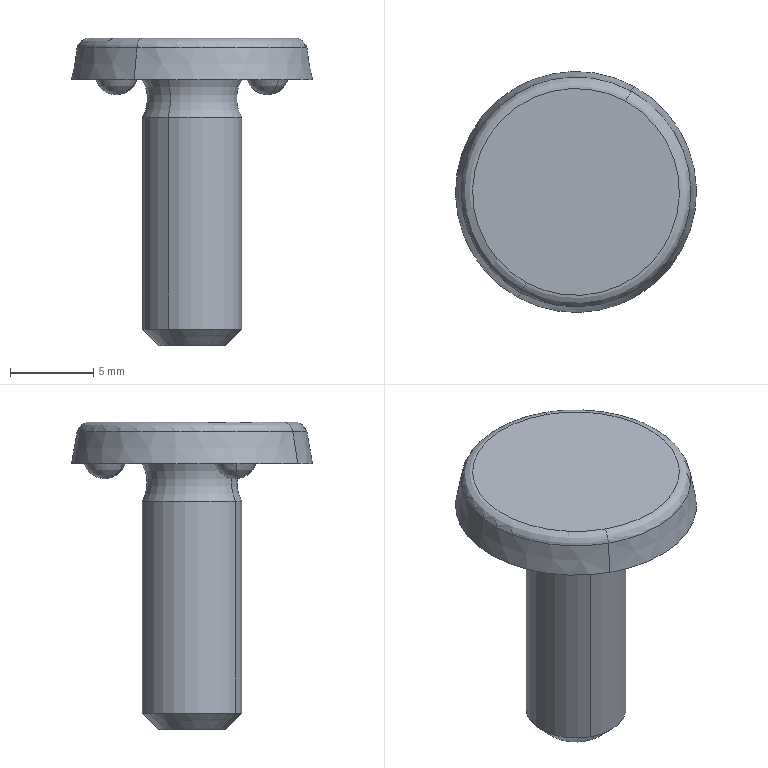Part | STEP file | Q1980616 | 1 solid | 19 faces | box 14.5 x 14.5 x 18.5 mm | volume 828.674 mm3 | sphere 6 | cone 4 | torus 4 | plane 3 | cylinder 2 | commonest cylinder face diameters 6 x2
STEP:
#1=CARTESIAN_POINT('',(4.547,-2.625,-0.9));
#2=VERTEX_POINT('',#1);
#3=CARTESIAN_POINT('',(5.19,-3.681,0.));
#4=VERTEX_POINT('',#3);
#5=CARTESIAN_POINT('',(4.547,-2.625,0.4));
#6=DIRECTION('',(0.854,0.5203,0.));
#7=AXIS2_PLACEMENT_3D('',#5,#6,$);
#8=CIRCLE('',#7,1.3);
#9=EDGE_CURVE('',#2,#4,#8,.F.);
#10=ORIENTED_EDGE('',*,*,#9,.F.);
#11=CARTESIAN_POINT('',(3.903,-1.569,0.));
#12=VERTEX_POINT('',#11);
#13=CARTESIAN_POINT('',(4.547,-2.625,0.4));
#14=DIRECTION('',(-0.854,-0.5203,0.));
#15=AXIS2_PLACEMENT_3D('',#13,#14,$);
#16=CIRCLE('',#15,1.3);
#17=EDGE_CURVE('',#2,#12,#16,.F.);
#18=ORIENTED_EDGE('',*,*,#17,.T.);
#19=CARTESIAN_POINT('',(5.19,-3.681,0.));
#20=CARTESIAN_POINT('',(5.46,-3.517,0.));
#21=CARTESIAN_POINT('',(5.678,-3.266,0.));
#22=CARTESIAN_POINT('',(5.805,-2.951,0.));
#23=CARTESIAN_POINT('',(5.832,-2.453,0.));
#24=CARTESIAN_POINT('',(5.639,-2.013,0.));
#25=CARTESIAN_POINT('',(5.551,-1.877,0.));
#26=CARTESIAN_POINT('',(5.238,-1.532,0.));
#27=CARTESIAN_POINT('',(4.79,-1.354,0.));
#28=CARTESIAN_POINT('',(4.468,-1.333,0.));
#29=CARTESIAN_POINT('',(4.161,-1.411,0.));
#30=CARTESIAN_POINT('',(3.903,-1.569,0.));
#31=B_SPLINE_CURVE_WITH_KNOTS('',5,(#19,#20,#21,#22,#23,#24,#25,#26,#27,#28,#29,#30),.UNSPECIFIED.,.F.,.U.,(6,3,3,6),(0.,2.294,3.444,5.637),.UNSPECIFIED.);
#32=EDGE_CURVE('',#4,#12,#31,.T.);
#33=ORIENTED_EDGE('',*,*,#32,.F.);
#34=EDGE_LOOP('',(#10,#18,#33));
#35=FACE_OUTER_BOUND('',#34,.T.);
#36=CARTESIAN_POINT('',(4.547,-2.625,0.4));
#37=DIRECTION('',(0.,0.,-1.));
#38=DIRECTION('',(0.5203,-0.854,0.));
#39=AXIS2_PLACEMENT_3D('',#36,#37,#38);
#40=SPHERICAL_SURFACE('',#39,1.3);
#41=ADVANCED_FACE('',(#35),#40,.T.);
#42=ORIENTED_EDGE('',*,*,#17,.F.);
#43=ORIENTED_EDGE('',*,*,#9,.T.);
#44=CARTESIAN_POINT('',(5.19,-3.681,0.));
#45=CARTESIAN_POINT('',(4.92,-3.846,0.));
#46=CARTESIAN_POINT('',(4.598,-3.924,0.));
#47=CARTESIAN_POINT('',(4.259,-3.893,0.));
#48=CARTESIAN_POINT('',(3.804,-3.689,0.));
#49=CARTESIAN_POINT('',(3.502,-3.315,0.));
#50=CARTESIAN_POINT('',(3.422,-3.175,0.));
#51=CARTESIAN_POINT('',(3.258,-2.738,0.));
#52=CARTESIAN_POINT('',(3.305,-2.258,0.));
#53=CARTESIAN_POINT('',(3.435,-1.962,0.));
#54=CARTESIAN_POINT('',(3.645,-1.726,0.));
#55=CARTESIAN_POINT('',(3.903,-1.569,0.));
#56=B_SPLINE_CURVE_WITH_KNOTS('',5,(#44,#45,#46,#47,#48,#49,#50,#51,#52,#53,#54,#55),.UNSPECIFIED.,.F.,.U.,(6,3,3,6),(0.,2.294,3.444,5.637),.UNSPECIFIED.);
#57=EDGE_CURVE('',#4,#12,#56,.T.);
#58=ORIENTED_EDGE('',*,*,#57,.T.);
#59=EDGE_LOOP('',(#42,#43,#58));
#60=FACE_OUTER_BOUND('',#59,.T.);
#61=ADVANCED_FACE('',(#60),#40,.T.);
#62=CARTESIAN_POINT('',(-3.476,-6.362,0.));
#63=VERTEX_POINT('',#62);
#64=CARTESIAN_POINT('',(3.476,6.362,0.));
#65=VERTEX_POINT('',#64);
#66=CARTESIAN_POINT('',(0.,0.,0.));
#67=DIRECTION('',(0.,0.,-1.));
#68=AXIS2_PLACEMENT_3D('',#66,#67,$);
#69=CIRCLE('',#68,7.25);
#70=EDGE_CURVE('',#63,#65,#69,.T.);
#71=ORIENTED_EDGE('',*,*,#70,.T.);
#72=CARTESIAN_POINT('',(0.,0.,0.));
#73=DIRECTION('',(0.,0.,-1.));
#74=AXIS2_PLACEMENT_3D('',#72,#73,$);
#75=CIRCLE('',#74,7.25);
#76=EDGE_CURVE('',#65,#63,#75,.T.);
#77=ORIENTED_EDGE('',*,*,#76,.T.);
#78=EDGE_LOOP('',(#71,#77));
#79=FACE_OUTER_BOUND('',#78,.T.);
#80=CARTESIAN_POINT('',(1.438,2.633,0.));
#81=VERTEX_POINT('',#80);
#82=CARTESIAN_POINT('',(-1.438,-2.633,0.));
#83=VERTEX_POINT('',#82);
#84=CARTESIAN_POINT('',(0.,0.,0.));
#85=DIRECTION('',(0.,0.,-1.));
#86=AXIS2_PLACEMENT_3D('',#84,#85,$);
#87=CIRCLE('',#86,3.);
#88=EDGE_CURVE('',#81,#83,#87,.T.);
#89=ORIENTED_EDGE('',*,*,#88,.F.);
#90=CARTESIAN_POINT('',(0.,0.,0.));
#91=DIRECTION('',(0.,0.,-1.));
#92=AXIS2_PLACEMENT_3D('',#90,#91,$);
#93=CIRCLE('',#92,3.);
#94=EDGE_CURVE('',#83,#81,#93,.T.);
#95=ORIENTED_EDGE('',*,*,#94,.F.);
#96=EDGE_LOOP('',(#89,#95));
#97=FACE_BOUND('',#96,.T.);
#98=CARTESIAN_POINT('',(-5.783,-2.654,0.));
#99=VERTEX_POINT('',#98);
#100=CARTESIAN_POINT('',(-3.31,-2.596,0.));
#101=VERTEX_POINT('',#100);
#102=CARTESIAN_POINT('',(-5.783,-2.654,0.));
#103=CARTESIAN_POINT('',(-5.787,-2.497,0.));
#104=CARTESIAN_POINT('',(-5.766,-2.338,0.));
#105=CARTESIAN_POINT('',(-5.719,-2.185,0.));
#106=CARTESIAN_POINT('',(-5.578,-1.897,0.));
#107=CARTESIAN_POINT('',(-5.355,-1.668,0.));
#108=CARTESIAN_POINT('',(-5.225,-1.572,0.));
#109=CARTESIAN_POINT('',(-4.939,-1.425,0.));
#110=CARTESIAN_POINT('',(-4.622,-1.375,0.));
#111=CARTESIAN_POINT('',(-4.46,-1.376,0.));
#112=CARTESIAN_POINT('',(-4.144,-1.429,0.));
#113=CARTESIAN_POINT('',(-3.859,-1.578,0.));
#114=CARTESIAN_POINT('',(-3.73,-1.675,0.));
#115=CARTESIAN_POINT('',(-3.519,-1.896,0.));
#116=CARTESIAN_POINT('',(-3.383,-2.17,0.));
#117=CARTESIAN_POINT('',(-3.338,-2.309,0.));
#118=CARTESIAN_POINT('',(-3.313,-2.452,0.));
#119=CARTESIAN_POINT('',(-3.31,-2.596,0.));
#120=B_SPLINE_CURVE_WITH_KNOTS('',5,(#102,#103,#104,#105,#106,#107,#108,#109,#110,#111,#112,#113,#114,#115,#116,#117,#118,#119),.UNSPECIFIED.,.F.,.U.,(6,3,3,3,3,6),(0.,1.143,2.294,3.444,4.595,5.637),.UNSPECIFIED.);
#121=EDGE_CURVE('',#99,#101,#120,.T.);
#122=ORIENTED_EDGE('',*,*,#121,.F.);
#123=CARTESIAN_POINT('',(-5.783,-2.654,0.));
#124=CARTESIAN_POINT('',(-5.78,-2.812,0.));
#125=CARTESIAN_POINT('',(-5.751,-2.969,0.));
#126=CARTESIAN_POINT('',(-5.697,-3.12,0.));
#127=CARTESIAN_POINT('',(-5.543,-3.4,0.));
#128=CARTESIAN_POINT('',(-5.309,-3.619,0.));
#129=CARTESIAN_POINT('',(-5.174,-3.709,0.));
#130=CARTESIAN_POINT('',(-4.882,-3.842,0.));
#131=CARTESIAN_POINT('',(-4.563,-3.877,0.));
#132=CARTESIAN_POINT('',(-4.402,-3.869,0.));
#133=CARTESIAN_POINT('',(-4.088,-3.801,0.));
#134=CARTESIAN_POINT('',(-3.811,-3.638,0.));
#135=CARTESIAN_POINT('',(-3.686,-3.535,0.));
#136=CARTESIAN_POINT('',(-3.485,-3.304,0.));
#137=CARTESIAN_POINT('',(-3.363,-3.024,0.));
#138=CARTESIAN_POINT('',(-3.324,-2.884,0.));
#139=CARTESIAN_POINT('',(-3.307,-2.74,0.));
#140=CARTESIAN_POINT('',(-3.31,-2.596,0.));
#141=B_SPLINE_CURVE_WITH_KNOTS('',5,(#123,#124,#125,#126,#127,#128,#129,#130,#131,#132,#133,#134,#135,#136,#137,#138,#139,#140),.UNSPECIFIED.,.F.,.U.,(6,3,3,3,3,6),(0.,1.143,2.294,3.444,4.595,5.637),.UNSPECIFIED.);
#142=EDGE_CURVE('',#99,#101,#141,.T.);
#143=ORIENTED_EDGE('',*,*,#142,.T.);
#144=EDGE_LOOP('',(#122,#143));
#145=FACE_BOUND('',#144,.T.);
#146=CARTESIAN_POINT('',(0.593,6.336,0.));
#147=VERTEX_POINT('',#146);
#148=CARTESIAN_POINT('',(-0.593,4.164,0.));
#149=VERTEX_POINT('',#148);
#150=CARTESIAN_POINT('',(0.593,6.336,0.));
#151=CARTESIAN_POINT('',(0.7313,6.26,0.));
#152=CARTESIAN_POINT('',(0.8576,6.162,0.));
#153=CARTESIAN_POINT('',(0.9672,6.045,0.));
#154=CARTESIAN_POINT('',(1.146,5.779,0.));
#155=CARTESIAN_POINT('',(1.233,5.471,0.));
#156=CARTESIAN_POINT('',(1.251,5.311,0.));
#157=CARTESIAN_POINT('',(1.235,4.99,0.));
#158=CARTESIAN_POINT('',(1.12,4.69,0.));
#159=CARTESIAN_POINT('',(1.039,4.551,0.));
#160=CARTESIAN_POINT('',(0.8345,4.303,0.));
#161=CARTESIAN_POINT('',(0.5629,4.131,0.));
#162=CARTESIAN_POINT('',(0.4143,4.068,0.));
#163=CARTESIAN_POINT('',(0.1169,3.995,0.));
#164=CARTESIAN_POINT('',(-0.188,4.015,0.));
#165=CARTESIAN_POINT('',(-0.3307,4.045,0.));
#166=CARTESIAN_POINT('',(-0.4669,4.096,0.));
#167=CARTESIAN_POINT('',(-0.593,4.164,0.));
#168=B_SPLINE_CURVE_WITH_KNOTS('',5,(#150,#151,#152,#153,#154,#155,#156,#157,#158,#159,#160,#161,#162,#163,#164,#165,#166,#167),.UNSPECIFIED.,.F.,.U.,(6,3,3,3,3,6),(0.,1.143,2.294,3.444,4.595,5.637),.UNSPECIFIED.);
#169=EDGE_CURVE('',#147,#149,#168,.T.);
#170=ORIENTED_EDGE('',*,*,#169,.F.);
#171=CARTESIAN_POINT('',(0.593,6.336,0.));
#172=CARTESIAN_POINT('',(0.4547,6.411,0.));
#173=CARTESIAN_POINT('',(0.3043,6.465,0.));
#174=CARTESIAN_POINT('',(0.1466,6.494,0.));
#175=CARTESIAN_POINT('',(-0.1735,6.5,0.));
#176=CARTESIAN_POINT('',(-0.4798,6.407,0.));
#177=CARTESIAN_POINT('',(-0.6246,6.335,0.));
#178=CARTESIAN_POINT('',(-0.8862,6.149,0.));
#179=CARTESIAN_POINT('',(-1.076,5.89,0.));
#180=CARTESIAN_POINT('',(-1.15,5.746,0.));
#181=CARTESIAN_POINT('',(-1.248,5.44,0.));
#182=CARTESIAN_POINT('',(-1.245,5.119,0.));
#183=CARTESIAN_POINT('',(-1.218,4.96,0.));
#184=CARTESIAN_POINT('',(-1.119,4.67,0.));
#185=CARTESIAN_POINT('',(-0.9379,4.424,0.));
#186=CARTESIAN_POINT('',(-0.8353,4.321,0.));
#187=CARTESIAN_POINT('',(-0.7192,4.233,0.));
#188=CARTESIAN_POINT('',(-0.593,4.164,0.));
#189=B_SPLINE_CURVE_WITH_KNOTS('',5,(#171,#172,#173,#174,#175,#176,#177,#178,#179,#180,#181,#182,#183,#184,#185,#186,#187,#188),.UNSPECIFIED.,.F.,.U.,(6,3,3,3,3,6),(0.,1.143,2.294,3.444,4.595,5.637),.UNSPECIFIED.);
#190=EDGE_CURVE('',#147,#149,#189,.T.);
#191=ORIENTED_EDGE('',*,*,#190,.T.);
#192=EDGE_LOOP('',(#170,#191));
#193=FACE_BOUND('',#192,.T.);
#194=ORIENTED_EDGE('',*,*,#57,.F.);
#195=ORIENTED_EDGE('',*,*,#32,.T.);
#196=EDGE_LOOP('',(#194,#195));
#197=FACE_BOUND('',#196,.T.);
#198=CARTESIAN_POINT('',(0.,3.,0.));
#199=DIRECTION('',(0.,0.,-1.));
#200=DIRECTION('',(1.,0.,0.));
#201=AXIS2_PLACEMENT_3D('',#198,#199,#200);
#202=PLANE('',#201);
#203=ADVANCED_FACE('',(#79,#97,#145,#193,#197),#202,.T.);
#204=ORIENTED_EDGE('',*,*,#70,.F.);
#205=CARTESIAN_POINT('',(-3.313,-6.065,1.922));
#206=VERTEX_POINT('',#205);
#207=CARTESIAN_POINT('',(-3.395,-6.214,0.9608));
#208=DIRECTION('',(-0.08325,-0.1524,-0.9848));
#209=VECTOR('',#208,1.);
#210=LINE('',#207,#209);
#211=EDGE_CURVE('',#63,#206,#210,.F.);
#212=ORIENTED_EDGE('',*,*,#211,.T.);
#213=CARTESIAN_POINT('',(3.313,6.065,1.922));
#214=VERTEX_POINT('',#213);
#215=CARTESIAN_POINT('',(0.,0.,1.922));
#216=DIRECTION('',(0.,0.,-1.));
#217=AXIS2_PLACEMENT_3D('',#215,#216,$);
#218=CIRCLE('',#217,6.911);
#219=EDGE_CURVE('',#206,#214,#218,.T.);
#220=ORIENTED_EDGE('',*,*,#219,.T.);
#221=CARTESIAN_POINT('',(3.395,6.214,0.9608));
#222=DIRECTION('',(0.08325,0.1524,-0.9848));
#223=VECTOR('',#222,1.);
#224=LINE('',#221,#223);
#225=EDGE_CURVE('',#65,#214,#224,.F.);
#226=ORIENTED_EDGE('',*,*,#225,.F.);
#227=EDGE_LOOP('',(#204,#212,#220,#226));
#228=FACE_OUTER_BOUND('',#227,.T.);
#229=CARTESIAN_POINT('',(0.,0.,1.922));
#230=DIRECTION('',(0.,0.,-1.));
#231=DIRECTION('',(0.4794,0.8776,0.));
#232=AXIS2_PLACEMENT_3D('',#229,#230,#231);
#233=CONICAL_SURFACE('',#232,6.911,0.1745);
#234=ADVANCED_FACE('',(#228),#233,.T.);
#235=ORIENTED_EDGE('',*,*,#76,.F.);
#236=ORIENTED_EDGE('',*,*,#225,.T.);
#237=CARTESIAN_POINT('',(0.,0.,1.922));
#238=DIRECTION('',(0.,0.,-1.));
#239=AXIS2_PLACEMENT_3D('',#237,#238,$);
#240=CIRCLE('',#239,6.911);
#241=EDGE_CURVE('',#214,#206,#240,.T.);
#242=ORIENTED_EDGE('',*,*,#241,.T.);
#243=ORIENTED_EDGE('',*,*,#211,.F.);
#244=EDGE_LOOP('',(#235,#236,#242,#243));
#245=FACE_OUTER_BOUND('',#244,.T.);
#246=ADVANCED_FACE('',(#245),#233,.T.);
#247=CARTESIAN_POINT('',(1.438,2.633,-2.25));
#248=VERTEX_POINT('',#247);
#249=CARTESIAN_POINT('',(-1.438,-2.633,-2.25));
#250=VERTEX_POINT('',#249);
#251=CARTESIAN_POINT('',(0.,0.,-2.25));
#252=DIRECTION('',(0.,0.,-1.));
#253=AXIS2_PLACEMENT_3D('',#251,#252,$);
#254=CIRCLE('',#253,3.);
#255=EDGE_CURVE('',#248,#250,#254,.T.);
#256=ORIENTED_EDGE('',*,*,#255,.F.);
#257=CARTESIAN_POINT('',(2.372,4.343,-1.125));
#258=DIRECTION('',(-0.8776,0.4794,0.));
#259=AXIS2_PLACEMENT_3D('',#257,#258,$);
#260=CIRCLE('',#259,2.25);
#261=EDGE_CURVE('',#248,#81,#260,.T.);
#262=ORIENTED_EDGE('',*,*,#261,.T.);
#263=ORIENTED_EDGE('',*,*,#88,.T.);
#264=CARTESIAN_POINT('',(-2.372,-4.343,-1.125));
#265=DIRECTION('',(0.8776,-0.4794,0.));
#266=AXIS2_PLACEMENT_3D('',#264,#265,$);
#267=CIRCLE('',#266,2.25);
#268=EDGE_CURVE('',#250,#83,#267,.T.);
#269=ORIENTED_EDGE('',*,*,#268,.F.);
#270=EDGE_LOOP('',(#256,#262,#263,#269));
#271=FACE_OUTER_BOUND('',#270,.T.);
#272=CARTESIAN_POINT('',(0.,0.,-1.125));
#273=DIRECTION('',(0.,0.,-1.));
#274=DIRECTION('',(0.4794,0.8776,0.));
#275=AXIS2_PLACEMENT_3D('',#272,#273,#274);
#276=TOROIDAL_SURFACE('',#275,4.949,2.25);
#277=ADVANCED_FACE('',(#271),#276,.F.);
#278=CARTESIAN_POINT('',(0.,0.,-2.25));
#279=DIRECTION('',(0.,0.,-1.));
#280=AXIS2_PLACEMENT_3D('',#278,#279,$);
#281=CIRCLE('',#280,3.);
#282=EDGE_CURVE('',#250,#248,#281,.T.);
#283=ORIENTED_EDGE('',*,*,#282,.F.);
#284=ORIENTED_EDGE('',*,*,#268,.T.);
#285=ORIENTED_EDGE('',*,*,#94,.T.);
#286=ORIENTED_EDGE('',*,*,#261,.F.);
#287=EDGE_LOOP('',(#283,#284,#285,#286));
#288=FACE_OUTER_BOUND('',#287,.T.);
#289=ADVANCED_FACE('',(#288),#276,.F.);
#290=CARTESIAN_POINT('',(-4.547,-2.625,-0.9));
#291=VERTEX_POINT('',#290);
#292=CARTESIAN_POINT('',(-4.547,-2.625,0.4));
#293=DIRECTION('',(-0.0236,0.9997,0.));
#294=AXIS2_PLACEMENT_3D('',#292,#293,$);
#295=CIRCLE('',#294,1.3);
#296=EDGE_CURVE('',#291,#101,#295,.F.);
#297=ORIENTED_EDGE('',*,*,#296,.F.);
#298=CARTESIAN_POINT('',(-4.547,-2.625,0.4));
#299=DIRECTION('',(0.0236,-0.9997,0.));
#300=AXIS2_PLACEMENT_3D('',#298,#299,$);
#301=CIRCLE('',#300,1.3);
#302=EDGE_CURVE('',#291,#99,#301,.F.);
#303=ORIENTED_EDGE('',*,*,#302,.T.);
#304=ORIENTED_EDGE('',*,*,#121,.T.);
#305=EDGE_LOOP('',(#297,#303,#304));
#306=FACE_OUTER_BOUND('',#305,.T.);
#307=CARTESIAN_POINT('',(-4.547,-2.625,0.4));
#308=DIRECTION('',(0.,0.,-1.));
#309=DIRECTION('',(-0.9997,-0.0236,0.));
#310=AXIS2_PLACEMENT_3D('',#307,#308,#309);
#311=SPHERICAL_SURFACE('',#310,1.3);
#312=ADVANCED_FACE('',(#306),#311,.T.);
#313=ORIENTED_EDGE('',*,*,#302,.F.);
#314=ORIENTED_EDGE('',*,*,#296,.T.);
#315=ORIENTED_EDGE('',*,*,#142,.F.);
#316=EDGE_LOOP('',(#313,#314,#315));
#317=FACE_OUTER_BOUND('',#316,.T.);
#318=ADVANCED_FACE('',(#317),#311,.T.);
#319=CARTESIAN_POINT('',(0.,5.25,-0.9));
#320=VERTEX_POINT('',#319);
#321=CARTESIAN_POINT('',(0.,5.25,0.4));
#322=DIRECTION('',(0.8776,-0.4794,0.));
#323=AXIS2_PLACEMENT_3D('',#321,#322,$);
#324=CIRCLE('',#323,1.3);
#325=EDGE_CURVE('',#320,#149,#324,.F.);
#326=ORIENTED_EDGE('',*,*,#325,.F.);
#327=CARTESIAN_POINT('',(0.,5.25,0.4));
#328=DIRECTION('',(-0.8776,0.4794,0.));
#329=AXIS2_PLACEMENT_3D('',#327,#328,$);
#330=CIRCLE('',#329,1.3);
#331=EDGE_CURVE('',#320,#147,#330,.F.);
#332=ORIENTED_EDGE('',*,*,#331,.T.);
#333=ORIENTED_EDGE('',*,*,#169,.T.);
#334=EDGE_LOOP('',(#326,#332,#333));
#335=FACE_OUTER_BOUND('',#334,.T.);
#336=CARTESIAN_POINT('',(0.,5.25,0.4));
#337=DIRECTION('',(0.,0.,-1.));
#338=DIRECTION('',(0.4794,0.8776,0.));
#339=AXIS2_PLACEMENT_3D('',#336,#337,#338);
#340=SPHERICAL_SURFACE('',#339,1.3);
#341=ADVANCED_FACE('',(#335),#340,.T.);
#342=ORIENTED_EDGE('',*,*,#331,.F.);
#343=ORIENTED_EDGE('',*,*,#325,.T.);
#344=ORIENTED_EDGE('',*,*,#190,.F.);
#345=EDGE_LOOP('',(#342,#343,#344));
#346=FACE_OUTER_BOUND('',#345,.T.);
#347=ADVANCED_FACE('',(#346),#340,.T.);
#348=ORIENTED_EDGE('',*,*,#219,.F.);
#349=CARTESIAN_POINT('',(-2.983,-5.46,2.5));
#350=VERTEX_POINT('',#349);
#351=CARTESIAN_POINT('',(-2.983,-5.46,1.8));
#352=DIRECTION('',(0.8776,-0.4794,0.));
#353=AXIS2_PLACEMENT_3D('',#351,#352,$);
#354=CIRCLE('',#353,0.7);
#355=EDGE_CURVE('',#206,#350,#354,.F.);
#356=ORIENTED_EDGE('',*,*,#355,.T.);
#357=CARTESIAN_POINT('',(2.983,5.46,2.5));
#358=VERTEX_POINT('',#357);
#359=CARTESIAN_POINT('',(0.,0.,2.5));
#360=DIRECTION('',(0.,0.,-1.));
#361=AXIS2_PLACEMENT_3D('',#359,#360,$);
#362=CIRCLE('',#361,6.222);
#363=EDGE_CURVE('',#350,#358,#362,.T.);
#364=ORIENTED_EDGE('',*,*,#363,.T.);
#365=CARTESIAN_POINT('',(2.983,5.46,1.8));
#366=DIRECTION('',(-0.8776,0.4794,0.));
#367=AXIS2_PLACEMENT_3D('',#365,#366,$);
#368=CIRCLE('',#367,0.7);
#369=EDGE_CURVE('',#214,#358,#368,.F.);
#370=ORIENTED_EDGE('',*,*,#369,.F.);
#371=EDGE_LOOP('',(#348,#356,#364,#370));
#372=FACE_OUTER_BOUND('',#371,.T.);
#373=CARTESIAN_POINT('',(0.,0.,1.8));
#374=DIRECTION('',(0.,0.,-1.));
#375=DIRECTION('',(0.4794,0.8776,0.));
#376=AXIS2_PLACEMENT_3D('',#373,#374,#375);
#377=TOROIDAL_SURFACE('',#376,6.222,0.7);
#378=ADVANCED_FACE('',(#372),#377,.T.);
#379=ORIENTED_EDGE('',*,*,#241,.F.);
#380=ORIENTED_EDGE('',*,*,#369,.T.);
#381=CARTESIAN_POINT('',(0.,0.,2.5));
#382=DIRECTION('',(0.,0.,-1.));
#383=AXIS2_PLACEMENT_3D('',#381,#382,$);
#384=CIRCLE('',#383,6.222);
#385=EDGE_CURVE('',#358,#350,#384,.T.);
#386=ORIENTED_EDGE('',*,*,#385,.T.);
#387=ORIENTED_EDGE('',*,*,#355,.F.);
#388=EDGE_LOOP('',(#379,#380,#386,#387));
#389=FACE_OUTER_BOUND('',#388,.T.);
#390=ADVANCED_FACE('',(#389),#377,.T.);
#391=CARTESIAN_POINT('',(1.438,2.633,-15.));
#392=VERTEX_POINT('',#391);
#393=CARTESIAN_POINT('',(-1.438,-2.633,-15.));
#394=VERTEX_POINT('',#393);
#395=CARTESIAN_POINT('',(0.,0.,-15.));
#396=DIRECTION('',(0.,0.,-1.));
#397=AXIS2_PLACEMENT_3D('',#395,#396,$);
#398=CIRCLE('',#397,3.);
#399=EDGE_CURVE('',#392,#394,#398,.T.);
#400=ORIENTED_EDGE('',*,*,#399,.F.);
#401=CARTESIAN_POINT('',(1.438,2.633,-8.625));
#402=DIRECTION('',(0.,0.,-1.));
#403=VECTOR('',#402,1.);
#404=LINE('',#401,#403);
#405=EDGE_CURVE('',#392,#248,#404,.F.);
#406=ORIENTED_EDGE('',*,*,#405,.T.);
#407=ORIENTED_EDGE('',*,*,#255,.T.);
#408=CARTESIAN_POINT('',(-1.438,-2.633,-8.625));
#409=DIRECTION('',(0.,0.,-1.));
#410=VECTOR('',#409,1.);
#411=LINE('',#408,#410);
#412=EDGE_CURVE('',#394,#250,#411,.F.);
#413=ORIENTED_EDGE('',*,*,#412,.F.);
#414=EDGE_LOOP('',(#400,#406,#407,#413));
#415=FACE_OUTER_BOUND('',#414,.T.);
#416=CARTESIAN_POINT('',(0.,0.,-6.75));
#417=DIRECTION('',(0.,0.,-1.));
#418=DIRECTION('',(0.4794,0.8776,0.));
#419=AXIS2_PLACEMENT_3D('',#416,#417,#418);
#420=CYLINDRICAL_SURFACE('',#419,3.);
#421=ADVANCED_FACE('',(#415),#420,.T.);
#422=CARTESIAN_POINT('',(0.,0.,-15.));
#423=DIRECTION('',(0.,0.,-1.));
#424=AXIS2_PLACEMENT_3D('',#422,#423,$);
#425=CIRCLE('',#424,3.);
#426=EDGE_CURVE('',#394,#392,#425,.T.);
#427=ORIENTED_EDGE('',*,*,#426,.F.);
#428=ORIENTED_EDGE('',*,*,#412,.T.);
#429=ORIENTED_EDGE('',*,*,#282,.T.);
#430=ORIENTED_EDGE('',*,*,#405,.F.);
#431=EDGE_LOOP('',(#427,#428,#429,#430));
#432=FACE_OUTER_BOUND('',#431,.T.);
#433=ADVANCED_FACE('',(#432),#420,.T.);
#434=ORIENTED_EDGE('',*,*,#385,.F.);
#435=ORIENTED_EDGE('',*,*,#363,.F.);
#436=EDGE_LOOP('',(#434,#435));
#437=FACE_OUTER_BOUND('',#436,.T.);
#438=CARTESIAN_POINT('',(0.,6.222,2.5));
#439=DIRECTION('',(0.,0.,-1.));
#440=DIRECTION('',(1.,0.,0.));
#441=AXIS2_PLACEMENT_3D('',#438,#439,#440);
#442=PLANE('',#441);
#443=ADVANCED_FACE('',(#437),#442,.F.);
#444=CARTESIAN_POINT('',(0.9589,1.755,-16.));
#445=VERTEX_POINT('',#444);
#446=CARTESIAN_POINT('',(-0.9589,-1.755,-16.));
#447=VERTEX_POINT('',#446);
#448=CARTESIAN_POINT('',(0.,0.,-16.));
#449=DIRECTION('',(0.,0.,1.));
#450=AXIS2_PLACEMENT_3D('',#448,#449,$);
#451=CIRCLE('',#450,2.);
#452=EDGE_CURVE('',#445,#447,#451,.F.);
#453=ORIENTED_EDGE('',*,*,#452,.F.);
#454=CARTESIAN_POINT('',(1.199,2.194,-15.5));
#455=DIRECTION('',(0.339,0.6205,0.7071));
#456=VECTOR('',#455,1.);
#457=LINE('',#454,#456);
#458=EDGE_CURVE('',#445,#392,#457,.T.);
#459=ORIENTED_EDGE('',*,*,#458,.T.);
#460=ORIENTED_EDGE('',*,*,#399,.T.);
#461=CARTESIAN_POINT('',(-1.199,-2.194,-15.5));
#462=DIRECTION('',(-0.339,-0.6205,0.7071));
#463=VECTOR('',#462,1.);
#464=LINE('',#461,#463);
#465=EDGE_CURVE('',#447,#394,#464,.T.);
#466=ORIENTED_EDGE('',*,*,#465,.F.);
#467=EDGE_LOOP('',(#453,#459,#460,#466));
#468=FACE_OUTER_BOUND('',#467,.T.);
#469=CARTESIAN_POINT('',(0.,0.,-16.));
#470=DIRECTION('',(0.,0.,1.));
#471=DIRECTION('',(0.4794,0.8776,0.));
#472=AXIS2_PLACEMENT_3D('',#469,#470,#471);
#473=CONICAL_SURFACE('',#472,2.,0.7854);
#474=ADVANCED_FACE('',(#468),#473,.T.);
#475=CARTESIAN_POINT('',(0.,0.,-16.));
#476=DIRECTION('',(0.,0.,1.));
#477=AXIS2_PLACEMENT_3D('',#475,#476,$);
#478=CIRCLE('',#477,2.);
#479=EDGE_CURVE('',#447,#445,#478,.F.);
#480=ORIENTED_EDGE('',*,*,#479,.F.);
#481=ORIENTED_EDGE('',*,*,#465,.T.);
#482=ORIENTED_EDGE('',*,*,#426,.T.);
#483=ORIENTED_EDGE('',*,*,#458,.F.);
#484=EDGE_LOOP('',(#480,#481,#482,#483));
#485=FACE_OUTER_BOUND('',#484,.T.);
#486=ADVANCED_FACE('',(#485),#473,.T.);
#487=ORIENTED_EDGE('',*,*,#452,.T.);
#488=ORIENTED_EDGE('',*,*,#479,.T.);
#489=EDGE_LOOP('',(#487,#488));
#490=FACE_OUTER_BOUND('',#489,.T.);
#491=CARTESIAN_POINT('',(0.,0.,-16.));
#492=DIRECTION('',(0.,0.,-1.));
#493=DIRECTION('',(1.,0.,0.));
#494=AXIS2_PLACEMENT_3D('',#491,#492,#493);
#495=PLANE('',#494);
#496=ADVANCED_FACE('',(#490),#495,.T.);
#497=CLOSED_SHELL('',(#41,#61,#203,#234,#246,#277,#289,#312,#318,#341,#347,#378,#390,#421,#433,#443,#474,#486,#496));
#498=MANIFOLD_SOLID_BREP('',#497);
#499=(LENGTH_UNIT()NAMED_UNIT(*)SI_UNIT(.MILLI.,.METRE.));
#500=UNCERTAINTY_MEASURE_WITH_UNIT(LENGTH_MEASURE(0.005),#499,'','');
#501=(NAMED_UNIT(*)PLANE_ANGLE_UNIT()SI_UNIT($,.RADIAN.));
#502=(NAMED_UNIT(*)SI_UNIT($,.STERADIAN.)SOLID_ANGLE_UNIT());
#503=(GEOMETRIC_REPRESENTATION_CONTEXT(3)GLOBAL_UNCERTAINTY_ASSIGNED_CONTEXT((#500))GLOBAL_UNIT_ASSIGNED_CONTEXT((#499,#501,#502))REPRESENTATION_CONTEXT('',''));
#504=ADVANCED_BREP_SHAPE_REPRESENTATION('',(#498),#503);